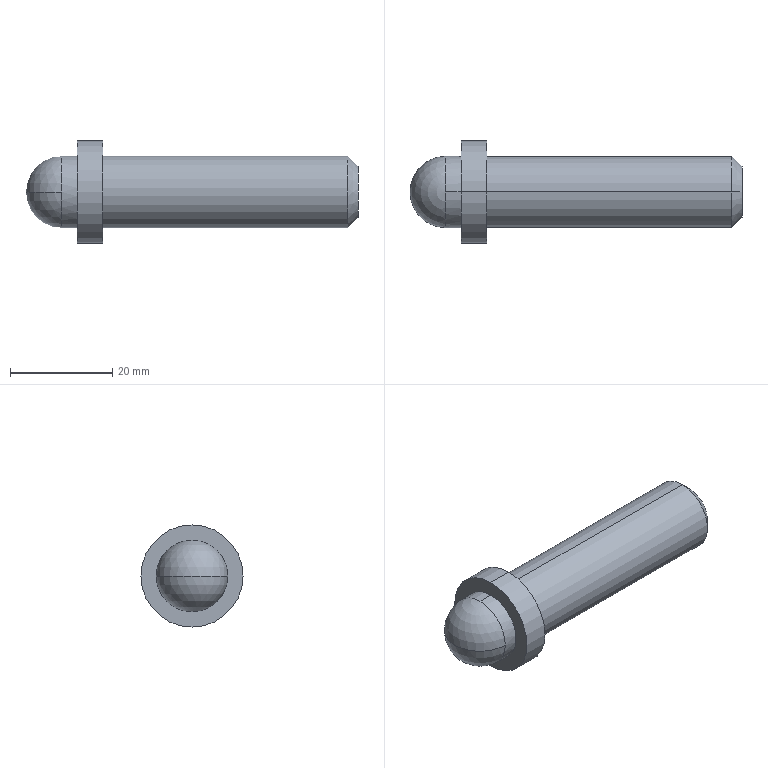Part | SolidWorks | features Revolution 1 | 1 solid | 13 faces | box 65 x 20 x 20 mm | volume 10368 mm3 | cylinder 6 | plane 3 | cone 2 | sphere 2 | commonest cylinder face diameters 14 x4 20 x2
STEP:
#1=CARTESIAN_POINT('',(0.,0.,5.));
#2=VERTEX_POINT('',#1);
#3=CARTESIAN_POINT('',(0.,0.,-5.));
#4=VERTEX_POINT('',#3);
#5=CARTESIAN_POINT('',(0.,0.,0.));
#6=DIRECTION('',(-1.,0.,0.));
#7=DIRECTION('',(0.,0.,1.));
#8=AXIS2_PLACEMENT_3D('',#5,#6,#7);
#9=CIRCLE('',#8,5.);
#10=EDGE_CURVE('',#2,#4,#9,.T.);
#11=ORIENTED_EDGE('',*,*,#10,.T.);
#12=CARTESIAN_POINT('',(-2.,0.,-7.));
#13=VERTEX_POINT('',#12);
#14=CARTESIAN_POINT('',(0.,0.,-5.));
#15=DIRECTION('',(-0.7071,0.,-0.7071));
#16=VECTOR('',#15,1000.);
#17=LINE('',#14,#16);
#18=EDGE_CURVE('',#4,#13,#17,.T.);
#19=ORIENTED_EDGE('',*,*,#18,.T.);
#20=CARTESIAN_POINT('',(-2.,0.,7.));
#21=VERTEX_POINT('',#20);
#22=CARTESIAN_POINT('',(-2.,0.,0.));
#23=DIRECTION('',(-1.,0.,0.));
#24=DIRECTION('',(0.,0.,1.));
#25=AXIS2_PLACEMENT_3D('',#22,#23,#24);
#26=CIRCLE('',#25,7.);
#27=EDGE_CURVE('',#21,#13,#26,.T.);
#28=ORIENTED_EDGE('',*,*,#27,.F.);
#29=CARTESIAN_POINT('',(0.,0.,5.));
#30=DIRECTION('',(-0.7071,0.,0.7071));
#31=VECTOR('',#30,1000.);
#32=LINE('',#29,#31);
#33=EDGE_CURVE('',#2,#21,#32,.T.);
#34=ORIENTED_EDGE('',*,*,#33,.F.);
#35=EDGE_LOOP('',(#11,#19,#28,#34));
#36=FACE_OUTER_BOUND('',#35,.T.);
#37=CARTESIAN_POINT('',(0.,0.,0.));
#38=DIRECTION('',(-1.,0.,0.));
#39=DIRECTION('',(0.,0.,1.));
#40=AXIS2_PLACEMENT_3D('',#37,#38,#39);
#41=CONICAL_SURFACE('',#40,5.,0.7854);
#42=ADVANCED_FACE('',(#36),#41,.T.);
#43=ORIENTED_EDGE('',*,*,#27,.T.);
#44=CARTESIAN_POINT('',(-50.,0.,-7.));
#45=VERTEX_POINT('',#44);
#46=CARTESIAN_POINT('',(-89.759,0.,-7.));
#47=DIRECTION('',(-1.,0.,0.));
#48=VECTOR('',#47,1000.);
#49=LINE('',#46,#48);
#50=EDGE_CURVE('',#13,#45,#49,.T.);
#51=ORIENTED_EDGE('',*,*,#50,.T.);
#52=CARTESIAN_POINT('',(-50.,0.,7.));
#53=VERTEX_POINT('',#52);
#54=CARTESIAN_POINT('',(-50.,0.,0.));
#55=DIRECTION('',(-1.,0.,0.));
#56=DIRECTION('',(0.,0.,1.));
#57=AXIS2_PLACEMENT_3D('',#54,#55,#56);
#58=CIRCLE('',#57,7.);
#59=EDGE_CURVE('',#53,#45,#58,.T.);
#60=ORIENTED_EDGE('',*,*,#59,.F.);
#61=CARTESIAN_POINT('',(-89.759,0.,7.));
#62=DIRECTION('',(-1.,0.,0.));
#63=VECTOR('',#62,1000.);
#64=LINE('',#61,#63);
#65=EDGE_CURVE('',#21,#53,#64,.T.);
#66=ORIENTED_EDGE('',*,*,#65,.F.);
#67=EDGE_LOOP('',(#43,#51,#60,#66));
#68=FACE_OUTER_BOUND('',#67,.T.);
#69=CARTESIAN_POINT('',(-89.759,0.,0.));
#70=DIRECTION('',(-1.,0.,0.));
#71=DIRECTION('',(0.,0.,1.));
#72=AXIS2_PLACEMENT_3D('',#69,#70,#71);
#73=CYLINDRICAL_SURFACE('',#72,7.);
#74=ADVANCED_FACE('',(#68),#73,.T.);
#75=CARTESIAN_POINT('',(-50.,0.,10.));
#76=VERTEX_POINT('',#75);
#77=CARTESIAN_POINT('',(-50.,0.,-10.));
#78=VERTEX_POINT('',#77);
#79=CARTESIAN_POINT('',(-50.,0.,0.));
#80=DIRECTION('',(-1.,0.,0.));
#81=DIRECTION('',(0.,0.,1.));
#82=AXIS2_PLACEMENT_3D('',#79,#80,#81);
#83=CIRCLE('',#82,10.);
#84=EDGE_CURVE('',#76,#78,#83,.T.);
#85=ORIENTED_EDGE('',*,*,#84,.T.);
#86=CARTESIAN_POINT('',(-55.,0.,-10.));
#87=VERTEX_POINT('',#86);
#88=CARTESIAN_POINT('',(-89.759,0.,-10.));
#89=DIRECTION('',(-1.,0.,0.));
#90=VECTOR('',#89,1000.);
#91=LINE('',#88,#90);
#92=EDGE_CURVE('',#78,#87,#91,.T.);
#93=ORIENTED_EDGE('',*,*,#92,.T.);
#94=CARTESIAN_POINT('',(-55.,0.,10.));
#95=VERTEX_POINT('',#94);
#96=CARTESIAN_POINT('',(-55.,0.,0.));
#97=DIRECTION('',(-1.,0.,0.));
#98=DIRECTION('',(0.,0.,1.));
#99=AXIS2_PLACEMENT_3D('',#96,#97,#98);
#100=CIRCLE('',#99,10.);
#101=EDGE_CURVE('',#95,#87,#100,.T.);
#102=ORIENTED_EDGE('',*,*,#101,.F.);
#103=CARTESIAN_POINT('',(-89.759,0.,10.));
#104=DIRECTION('',(-1.,0.,0.));
#105=VECTOR('',#104,1000.);
#106=LINE('',#103,#105);
#107=EDGE_CURVE('',#76,#95,#106,.T.);
#108=ORIENTED_EDGE('',*,*,#107,.F.);
#109=EDGE_LOOP('',(#85,#93,#102,#108));
#110=FACE_OUTER_BOUND('',#109,.T.);
#111=CARTESIAN_POINT('',(-89.759,0.,0.));
#112=DIRECTION('',(-1.,0.,0.));
#113=DIRECTION('',(0.,0.,1.));
#114=AXIS2_PLACEMENT_3D('',#111,#112,#113);
#115=CYLINDRICAL_SURFACE('',#114,10.);
#116=ADVANCED_FACE('',(#110),#115,.T.);
#117=CARTESIAN_POINT('',(-55.,0.,7.));
#118=VERTEX_POINT('',#117);
#119=CARTESIAN_POINT('',(-55.,0.,-7.));
#120=VERTEX_POINT('',#119);
#121=CARTESIAN_POINT('',(-55.,0.,0.));
#122=DIRECTION('',(-1.,0.,0.));
#123=DIRECTION('',(0.,0.,1.));
#124=AXIS2_PLACEMENT_3D('',#121,#122,#123);
#125=CIRCLE('',#124,7.);
#126=EDGE_CURVE('',#118,#120,#125,.T.);
#127=ORIENTED_EDGE('',*,*,#126,.T.);
#128=CARTESIAN_POINT('',(-58.,0.,-7.));
#129=VERTEX_POINT('',#128);
#130=CARTESIAN_POINT('',(-89.759,0.,-7.));
#131=DIRECTION('',(-1.,0.,0.));
#132=VECTOR('',#131,1000.);
#133=LINE('',#130,#132);
#134=EDGE_CURVE('',#120,#129,#133,.T.);
#135=ORIENTED_EDGE('',*,*,#134,.T.);
#136=CARTESIAN_POINT('',(-58.,7.,0.));
#137=VERTEX_POINT('',#136);
#138=CARTESIAN_POINT('',(-58.,0.,0.));
#139=DIRECTION('',(-1.,0.,0.));
#140=DIRECTION('',(0.,0.,1.));
#141=AXIS2_PLACEMENT_3D('',#138,#139,#140);
#142=CIRCLE('',#141,7.);
#143=EDGE_CURVE('',#137,#129,#142,.T.);
#144=ORIENTED_EDGE('',*,*,#143,.F.);
#145=CARTESIAN_POINT('',(-58.,0.,7.));
#146=VERTEX_POINT('',#145);
#147=CARTESIAN_POINT('',(-58.,0.,0.));
#148=DIRECTION('',(-1.,0.,0.));
#149=DIRECTION('',(0.,0.,1.));
#150=AXIS2_PLACEMENT_3D('',#147,#148,#149);
#151=CIRCLE('',#150,7.);
#152=EDGE_CURVE('',#146,#137,#151,.T.);
#153=ORIENTED_EDGE('',*,*,#152,.F.);
#154=CARTESIAN_POINT('',(-89.759,0.,7.));
#155=DIRECTION('',(-1.,0.,0.));
#156=VECTOR('',#155,1000.);
#157=LINE('',#154,#156);
#158=EDGE_CURVE('',#118,#146,#157,.T.);
#159=ORIENTED_EDGE('',*,*,#158,.F.);
#160=EDGE_LOOP('',(#127,#135,#144,#153,#159));
#161=FACE_OUTER_BOUND('',#160,.T.);
#162=CARTESIAN_POINT('',(-89.759,0.,0.));
#163=DIRECTION('',(-1.,0.,0.));
#164=DIRECTION('',(0.,0.,1.));
#165=AXIS2_PLACEMENT_3D('',#162,#163,#164);
#166=CYLINDRICAL_SURFACE('',#165,7.);
#167=ADVANCED_FACE('',(#161),#166,.T.);
#168=ORIENTED_EDGE('',*,*,#143,.T.);
#169=CARTESIAN_POINT('',(-58.,-7.,0.));
#170=VERTEX_POINT('',#169);
#171=CARTESIAN_POINT('',(-58.,0.,0.));
#172=DIRECTION('',(-1.,0.,0.));
#173=DIRECTION('',(0.,0.,1.));
#174=AXIS2_PLACEMENT_3D('',#171,#172,#173);
#175=CIRCLE('',#174,7.);
#176=EDGE_CURVE('',#129,#170,#175,.T.);
#177=ORIENTED_EDGE('',*,*,#176,.T.);
#178=CARTESIAN_POINT('',(-65.,0.,0.));
#179=VERTEX_POINT('',#178);
#180=CARTESIAN_POINT('',(-58.,0.,0.));
#181=DIRECTION('',(0.,0.,-1.));
#182=DIRECTION('',(0.,1.,0.));
#183=AXIS2_PLACEMENT_3D('',#180,#181,#182);
#184=CIRCLE('',#183,7.);
#185=EDGE_CURVE('',#170,#179,#184,.T.);
#186=ORIENTED_EDGE('',*,*,#185,.T.);
#187=CARTESIAN_POINT('',(-58.,0.,0.));
#188=DIRECTION('',(0.,0.,1.));
#189=DIRECTION('',(1.,0.,0.));
#190=AXIS2_PLACEMENT_3D('',#187,#188,#189);
#191=CIRCLE('',#190,7.);
#192=EDGE_CURVE('',#137,#179,#191,.T.);
#193=ORIENTED_EDGE('',*,*,#192,.F.);
#194=EDGE_LOOP('',(#168,#177,#186,#193));
#195=FACE_OUTER_BOUND('',#194,.T.);
#196=CARTESIAN_POINT('',(-58.,0.,0.));
#197=DIRECTION('',(0.,0.,-1.));
#198=DIRECTION('',(0.,1.,0.));
#199=AXIS2_PLACEMENT_3D('',#196,#197,#198);
#200=SPHERICAL_SURFACE('',#199,7.);
#201=ADVANCED_FACE('',(#195),#200,.T.);
#202=ORIENTED_EDGE('',*,*,#185,.F.);
#203=CARTESIAN_POINT('',(-58.,0.,0.));
#204=DIRECTION('',(-1.,0.,0.));
#205=DIRECTION('',(0.,0.,1.));
#206=AXIS2_PLACEMENT_3D('',#203,#204,#205);
#207=CIRCLE('',#206,7.);
#208=EDGE_CURVE('',#170,#146,#207,.T.);
#209=ORIENTED_EDGE('',*,*,#208,.T.);
#210=ORIENTED_EDGE('',*,*,#152,.T.);
#211=ORIENTED_EDGE('',*,*,#192,.T.);
#212=EDGE_LOOP('',(#202,#209,#210,#211));
#213=FACE_OUTER_BOUND('',#212,.T.);
#214=CARTESIAN_POINT('',(-58.,0.,0.));
#215=DIRECTION('',(0.,0.,-1.));
#216=DIRECTION('',(0.,1.,0.));
#217=AXIS2_PLACEMENT_3D('',#214,#215,#216);
#218=SPHERICAL_SURFACE('',#217,7.);
#219=ADVANCED_FACE('',(#213),#218,.T.);
#220=ORIENTED_EDGE('',*,*,#134,.F.);
#221=CARTESIAN_POINT('',(-55.,0.,0.));
#222=DIRECTION('',(-1.,0.,0.));
#223=DIRECTION('',(0.,0.,1.));
#224=AXIS2_PLACEMENT_3D('',#221,#222,#223);
#225=CIRCLE('',#224,7.);
#226=EDGE_CURVE('',#120,#118,#225,.T.);
#227=ORIENTED_EDGE('',*,*,#226,.T.);
#228=ORIENTED_EDGE('',*,*,#158,.T.);
#229=ORIENTED_EDGE('',*,*,#208,.F.);
#230=ORIENTED_EDGE('',*,*,#176,.F.);
#231=EDGE_LOOP('',(#220,#227,#228,#229,#230));
#232=FACE_OUTER_BOUND('',#231,.T.);
#233=CARTESIAN_POINT('',(-89.759,0.,0.));
#234=DIRECTION('',(-1.,0.,0.));
#235=DIRECTION('',(0.,0.,1.));
#236=AXIS2_PLACEMENT_3D('',#233,#234,#235);
#237=CYLINDRICAL_SURFACE('',#236,7.);
#238=ADVANCED_FACE('',(#232),#237,.T.);
#239=ORIENTED_EDGE('',*,*,#126,.F.);
#240=ORIENTED_EDGE('',*,*,#226,.F.);
#241=EDGE_LOOP('',(#239,#240));
#242=FACE_BOUND('',#241,.T.);
#243=ORIENTED_EDGE('',*,*,#101,.T.);
#244=CARTESIAN_POINT('',(-55.,0.,0.));
#245=DIRECTION('',(-1.,0.,0.));
#246=DIRECTION('',(0.,0.,1.));
#247=AXIS2_PLACEMENT_3D('',#244,#245,#246);
#248=CIRCLE('',#247,10.);
#249=EDGE_CURVE('',#87,#95,#248,.T.);
#250=ORIENTED_EDGE('',*,*,#249,.T.);
#251=EDGE_LOOP('',(#243,#250));
#252=FACE_OUTER_BOUND('',#251,.T.);
#253=CARTESIAN_POINT('',(-55.,10.,0.));
#254=DIRECTION('',(1.,0.,0.));
#255=DIRECTION('',(0.,0.,-1.));
#256=AXIS2_PLACEMENT_3D('',#253,#254,#255);
#257=PLANE('',#256);
#258=ADVANCED_FACE('',(#242,#252),#257,.F.);
#259=ORIENTED_EDGE('',*,*,#92,.F.);
#260=CARTESIAN_POINT('',(-50.,0.,0.));
#261=DIRECTION('',(-1.,0.,0.));
#262=DIRECTION('',(0.,0.,1.));
#263=AXIS2_PLACEMENT_3D('',#260,#261,#262);
#264=CIRCLE('',#263,10.);
#265=EDGE_CURVE('',#78,#76,#264,.T.);
#266=ORIENTED_EDGE('',*,*,#265,.T.);
#267=ORIENTED_EDGE('',*,*,#107,.T.);
#268=ORIENTED_EDGE('',*,*,#249,.F.);
#269=EDGE_LOOP('',(#259,#266,#267,#268));
#270=FACE_OUTER_BOUND('',#269,.T.);
#271=CARTESIAN_POINT('',(-89.759,0.,0.));
#272=DIRECTION('',(-1.,0.,0.));
#273=DIRECTION('',(0.,0.,1.));
#274=AXIS2_PLACEMENT_3D('',#271,#272,#273);
#275=CYLINDRICAL_SURFACE('',#274,10.);
#276=ADVANCED_FACE('',(#270),#275,.T.);
#277=ORIENTED_EDGE('',*,*,#84,.F.);
#278=ORIENTED_EDGE('',*,*,#265,.F.);
#279=EDGE_LOOP('',(#277,#278));
#280=FACE_OUTER_BOUND('',#279,.T.);
#281=ORIENTED_EDGE('',*,*,#59,.T.);
#282=CARTESIAN_POINT('',(-50.,0.,0.));
#283=DIRECTION('',(-1.,0.,0.));
#284=DIRECTION('',(0.,0.,1.));
#285=AXIS2_PLACEMENT_3D('',#282,#283,#284);
#286=CIRCLE('',#285,7.);
#287=EDGE_CURVE('',#45,#53,#286,.T.);
#288=ORIENTED_EDGE('',*,*,#287,.T.);
#289=EDGE_LOOP('',(#281,#288));
#290=FACE_BOUND('',#289,.T.);
#291=CARTESIAN_POINT('',(-50.,7.,0.));
#292=DIRECTION('',(-1.,0.,0.));
#293=DIRECTION('',(0.,0.,1.));
#294=AXIS2_PLACEMENT_3D('',#291,#292,#293);
#295=PLANE('',#294);
#296=ADVANCED_FACE('',(#280,#290),#295,.F.);
#297=ORIENTED_EDGE('',*,*,#50,.F.);
#298=CARTESIAN_POINT('',(-2.,0.,0.));
#299=DIRECTION('',(-1.,0.,0.));
#300=DIRECTION('',(0.,0.,1.));
#301=AXIS2_PLACEMENT_3D('',#298,#299,#300);
#302=CIRCLE('',#301,7.);
#303=EDGE_CURVE('',#13,#21,#302,.T.);
#304=ORIENTED_EDGE('',*,*,#303,.T.);
#305=ORIENTED_EDGE('',*,*,#65,.T.);
#306=ORIENTED_EDGE('',*,*,#287,.F.);
#307=EDGE_LOOP('',(#297,#304,#305,#306));
#308=FACE_OUTER_BOUND('',#307,.T.);
#309=CARTESIAN_POINT('',(-89.759,0.,0.));
#310=DIRECTION('',(-1.,0.,0.));
#311=DIRECTION('',(0.,0.,1.));
#312=AXIS2_PLACEMENT_3D('',#309,#310,#311);
#313=CYLINDRICAL_SURFACE('',#312,7.);
#314=ADVANCED_FACE('',(#308),#313,.T.);
#315=ORIENTED_EDGE('',*,*,#18,.F.);
#316=CARTESIAN_POINT('',(0.,0.,0.));
#317=DIRECTION('',(-1.,0.,0.));
#318=DIRECTION('',(0.,0.,1.));
#319=AXIS2_PLACEMENT_3D('',#316,#317,#318);
#320=CIRCLE('',#319,5.);
#321=EDGE_CURVE('',#4,#2,#320,.T.);
#322=ORIENTED_EDGE('',*,*,#321,.T.);
#323=ORIENTED_EDGE('',*,*,#33,.T.);
#324=ORIENTED_EDGE('',*,*,#303,.F.);
#325=EDGE_LOOP('',(#315,#322,#323,#324));
#326=FACE_OUTER_BOUND('',#325,.T.);
#327=CARTESIAN_POINT('',(0.,0.,0.));
#328=DIRECTION('',(-1.,0.,0.));
#329=DIRECTION('',(0.,0.,1.));
#330=AXIS2_PLACEMENT_3D('',#327,#328,#329);
#331=CONICAL_SURFACE('',#330,5.,0.7854);
#332=ADVANCED_FACE('',(#326),#331,.T.);
#333=ORIENTED_EDGE('',*,*,#10,.F.);
#334=ORIENTED_EDGE('',*,*,#321,.F.);
#335=EDGE_LOOP('',(#333,#334));
#336=FACE_OUTER_BOUND('',#335,.T.);
#337=CARTESIAN_POINT('',(0.,0.,0.));
#338=DIRECTION('',(-1.,0.,0.));
#339=DIRECTION('',(0.,0.,1.));
#340=AXIS2_PLACEMENT_3D('',#337,#338,#339);
#341=PLANE('',#340);
#342=ADVANCED_FACE('',(#336),#341,.F.);
#343=CLOSED_SHELL('',(#42,#74,#116,#167,#201,#219,#238,#258,#276,#296,#314,#332,#342));
#344=MANIFOLD_SOLID_BREP('',#343);
#345=CARTESIAN_POINT('',(0.,0.,0.));
#346=DIRECTION('',(0.,0.,1.));
#347=DIRECTION('',(1.,0.,0.));
#348=AXIS2_PLACEMENT_3D('',#345,#346,#347);
#349=(LENGTH_UNIT()NAMED_UNIT(*)SI_UNIT(.MILLI.,.METRE.));
#350=UNCERTAINTY_MEASURE_WITH_UNIT(LENGTH_MEASURE(0.00001),#349,'','');
#351=(NAMED_UNIT(*)PLANE_ANGLE_UNIT()SI_UNIT($,.RADIAN.));
#352=(NAMED_UNIT(*)SI_UNIT($,.STERADIAN.)SOLID_ANGLE_UNIT());
#353=(GEOMETRIC_REPRESENTATION_CONTEXT(3)GLOBAL_UNCERTAINTY_ASSIGNED_CONTEXT((#350))GLOBAL_UNIT_ASSIGNED_CONTEXT((#349,#351,#352))REPRESENTATION_CONTEXT('',''));
#354=ADVANCED_BREP_SHAPE_REPRESENTATION('',(#344,#348),#353);